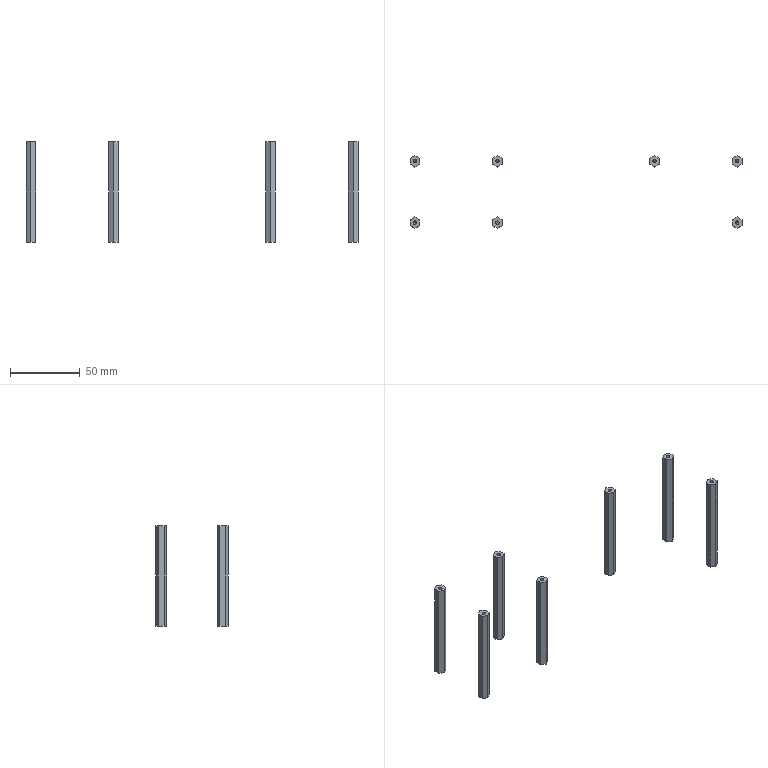Part | SolidWorks | features Extrusion 1, HoleWzd 1 | 7 solids | 84 faces | box 237.4 x 52 x 72 mm | volume 21087 mm3 | plane 56 | cylinder 14 | cone 14 | commonest cylinder face diameters 2.5 x14